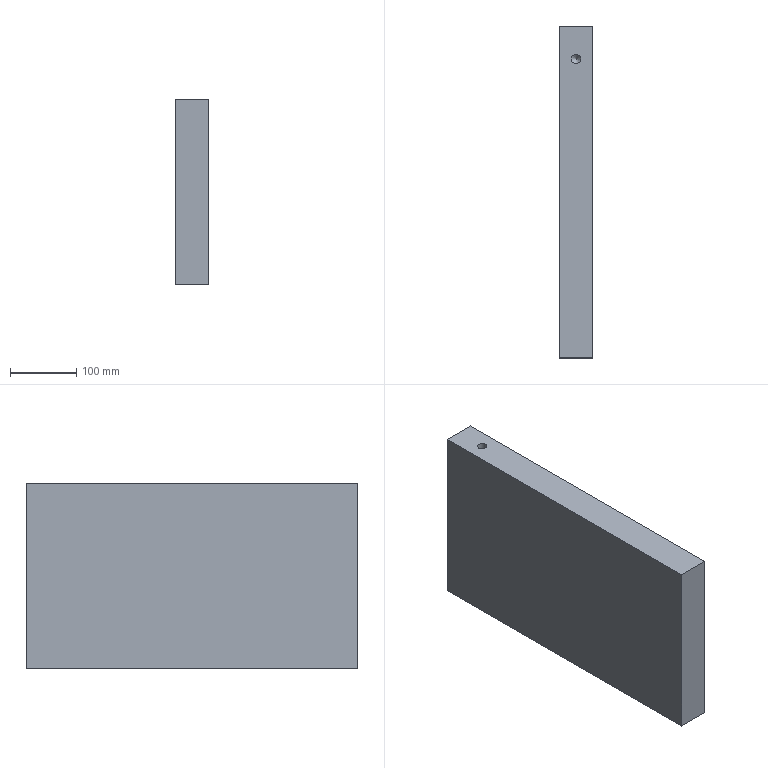Part | NX | features 29 2 | 1 solid | 12 faces | box 50 x 502.5 x 280.5 mm | volume 7029153 mm3 | plane 6 | cylinder 3 | cone 3 | commonest cylinder face diameters 14.1 x3
STEP:
#1=CARTESIAN_POINT('',(3262.05,622.5,-493.5));
#2=VERTEX_POINT('',#1);
#3=CARTESIAN_POINT('',(3255.,622.5,-493.5));
#4=DIRECTION('',(0.,0.,1.));
#5=DIRECTION('',(1.,0.,0.));
#6=AXIS2_PLACEMENT_3D('',#3,#4,#5);
#7=CIRCLE('',#6,7.05);
#8=EDGE_CURVE('',#2,#2,#7,.T.);
#9=ORIENTED_EDGE('',*,*,#8,.T.);
#10=EDGE_LOOP('',(#9));
#11=FACE_BOUND('',#10,.T.);
#12=CARTESIAN_POINT('',(3230.,170.,-493.5));
#13=VERTEX_POINT('',#12);
#14=CARTESIAN_POINT('',(3280.,170.,-493.5));
#15=VERTEX_POINT('',#14);
#16=CARTESIAN_POINT('',(1945.,170.,-493.5));
#17=DIRECTION('',(1.,0.,0.));
#18=VECTOR('',#17,1000.);
#19=LINE('',#16,#18);
#20=EDGE_CURVE('',#13,#15,#19,.T.);
#21=ORIENTED_EDGE('',*,*,#20,.F.);
#22=CARTESIAN_POINT('',(3230.,672.5,-493.5));
#23=VERTEX_POINT('',#22);
#24=CARTESIAN_POINT('',(3230.,193.,-493.5));
#25=DIRECTION('',(0.,-1.,0.));
#26=VECTOR('',#25,1000.);
#27=LINE('',#24,#26);
#28=EDGE_CURVE('',#23,#13,#27,.T.);
#29=ORIENTED_EDGE('',*,*,#28,.F.);
#30=CARTESIAN_POINT('',(3280.,672.5,-493.5));
#31=VERTEX_POINT('',#30);
#32=CARTESIAN_POINT('',(1117.5,672.5,-493.5));
#33=DIRECTION('',(1.,0.,0.));
#34=VECTOR('',#33,1000.);
#35=LINE('',#32,#34);
#36=EDGE_CURVE('',#23,#31,#35,.T.);
#37=ORIENTED_EDGE('',*,*,#36,.T.);
#38=CARTESIAN_POINT('',(3280.,193.,-493.5));
#39=DIRECTION('',(0.,1.,0.));
#40=VECTOR('',#39,1000.);
#41=LINE('',#38,#40);
#42=EDGE_CURVE('',#15,#31,#41,.T.);
#43=ORIENTED_EDGE('',*,*,#42,.F.);
#44=EDGE_LOOP('',(#21,#29,#37,#43));
#45=FACE_BOUND('',#44,.T.);
#46=CARTESIAN_POINT('',(3262.05,242.5,-493.5));
#47=VERTEX_POINT('',#46);
#48=CARTESIAN_POINT('',(3255.,242.5,-493.5));
#49=DIRECTION('',(0.,0.,1.));
#50=DIRECTION('',(1.,0.,0.));
#51=AXIS2_PLACEMENT_3D('',#48,#49,#50);
#52=CIRCLE('',#51,7.05);
#53=EDGE_CURVE('',#47,#47,#52,.T.);
#54=ORIENTED_EDGE('',*,*,#53,.T.);
#55=EDGE_LOOP('',(#54));
#56=FACE_BOUND('',#55,.T.);
#57=CARTESIAN_POINT('',(1945.,0.,-493.5));
#58=DIRECTION('',(0.,0.,-1.));
#59=DIRECTION('',(1.,0.,0.));
#60=AXIS2_PLACEMENT_3D('',#57,#58,#59);
#61=PLANE('',#60);
#62=ADVANCED_FACE('',(#11,#45,#56),#61,.T.);
#63=CARTESIAN_POINT('',(3230.,170.,-213.));
#64=VERTEX_POINT('',#63);
#65=CARTESIAN_POINT('',(3280.,170.,-213.));
#66=VERTEX_POINT('',#65);
#67=CARTESIAN_POINT('',(1945.,170.,-213.));
#68=DIRECTION('',(1.,0.,0.));
#69=VECTOR('',#68,1000.);
#70=LINE('',#67,#69);
#71=EDGE_CURVE('',#64,#66,#70,.T.);
#72=ORIENTED_EDGE('',*,*,#71,.T.);
#73=CARTESIAN_POINT('',(3280.,672.5,-213.));
#74=VERTEX_POINT('',#73);
#75=CARTESIAN_POINT('',(3280.,193.,-213.));
#76=DIRECTION('',(0.,-1.,0.));
#77=VECTOR('',#76,1000.);
#78=LINE('',#75,#77);
#79=EDGE_CURVE('',#74,#66,#78,.T.);
#80=ORIENTED_EDGE('',*,*,#79,.F.);
#81=CARTESIAN_POINT('',(3230.,672.5,-213.));
#82=VERTEX_POINT('',#81);
#83=CARTESIAN_POINT('',(1117.5,672.5,-213.));
#84=DIRECTION('',(-1.,0.,0.));
#85=VECTOR('',#84,1000.);
#86=LINE('',#83,#85);
#87=EDGE_CURVE('',#74,#82,#86,.T.);
#88=ORIENTED_EDGE('',*,*,#87,.T.);
#89=CARTESIAN_POINT('',(3230.,193.,-213.));
#90=DIRECTION('',(0.,1.,0.));
#91=VECTOR('',#90,1000.);
#92=LINE('',#89,#91);
#93=EDGE_CURVE('',#64,#82,#92,.T.);
#94=ORIENTED_EDGE('',*,*,#93,.F.);
#95=EDGE_LOOP('',(#72,#80,#88,#94));
#96=FACE_BOUND('',#95,.T.);
#97=CARTESIAN_POINT('',(3262.05,622.5,-213.));
#98=VERTEX_POINT('',#97);
#99=CARTESIAN_POINT('',(3255.,622.5,-213.));
#100=DIRECTION('',(0.,0.,-1.));
#101=DIRECTION('',(1.,0.,0.));
#102=AXIS2_PLACEMENT_3D('',#99,#100,#101);
#103=CIRCLE('',#102,7.05);
#104=EDGE_CURVE('',#98,#98,#103,.T.);
#105=ORIENTED_EDGE('',*,*,#104,.T.);
#106=EDGE_LOOP('',(#105));
#107=FACE_BOUND('',#106,.T.);
#108=CARTESIAN_POINT('',(1945.,0.,-213.));
#109=DIRECTION('',(0.,0.,1.));
#110=DIRECTION('',(-1.,0.,0.));
#111=AXIS2_PLACEMENT_3D('',#108,#109,#110);
#112=PLANE('',#111);
#113=ADVANCED_FACE('',(#96,#107),#112,.T.);
#114=CARTESIAN_POINT('',(3230.,170.,-205.5));
#115=DIRECTION('',(0.,0.,-1.));
#116=VECTOR('',#115,1000.);
#117=LINE('',#114,#116);
#118=EDGE_CURVE('',#64,#13,#117,.T.);
#119=ORIENTED_EDGE('',*,*,#118,.F.);
#120=ORIENTED_EDGE('',*,*,#93,.T.);
#121=CARTESIAN_POINT('',(3230.,672.5,-205.5));
#122=DIRECTION('',(0.,0.,1.));
#123=VECTOR('',#122,1000.);
#124=LINE('',#121,#123);
#125=EDGE_CURVE('',#23,#82,#124,.T.);
#126=ORIENTED_EDGE('',*,*,#125,.F.);
#127=ORIENTED_EDGE('',*,*,#28,.T.);
#128=EDGE_LOOP('',(#119,#120,#126,#127));
#129=FACE_BOUND('',#128,.T.);
#130=CARTESIAN_POINT('',(3230.,193.,-205.5));
#131=DIRECTION('',(-1.,0.,0.));
#132=DIRECTION('',(0.,0.,1.));
#133=AXIS2_PLACEMENT_3D('',#130,#131,#132);
#134=PLANE('',#133);
#135=ADVANCED_FACE('',(#129),#134,.T.);
#136=ORIENTED_EDGE('',*,*,#36,.F.);
#137=ORIENTED_EDGE('',*,*,#125,.T.);
#138=ORIENTED_EDGE('',*,*,#87,.F.);
#139=CARTESIAN_POINT('',(3280.,672.5,-205.5));
#140=DIRECTION('',(0.,0.,1.));
#141=VECTOR('',#140,1000.);
#142=LINE('',#139,#141);
#143=EDGE_CURVE('',#31,#74,#142,.T.);
#144=ORIENTED_EDGE('',*,*,#143,.F.);
#145=EDGE_LOOP('',(#136,#137,#138,#144));
#146=FACE_BOUND('',#145,.T.);
#147=CARTESIAN_POINT('',(1117.5,672.5,91.));
#148=DIRECTION('',(0.,-1.,0.));
#149=DIRECTION('',(-1.,0.,0.));
#150=AXIS2_PLACEMENT_3D('',#147,#148,#149);
#151=PLANE('',#150);
#152=ADVANCED_FACE('',(#146),#151,.F.);
#153=CARTESIAN_POINT('',(3280.,170.,-205.5));
#154=DIRECTION('',(0.,0.,-1.));
#155=VECTOR('',#154,1000.);
#156=LINE('',#153,#155);
#157=EDGE_CURVE('',#66,#15,#156,.T.);
#158=ORIENTED_EDGE('',*,*,#157,.T.);
#159=ORIENTED_EDGE('',*,*,#42,.T.);
#160=ORIENTED_EDGE('',*,*,#143,.T.);
#161=ORIENTED_EDGE('',*,*,#79,.T.);
#162=EDGE_LOOP('',(#158,#159,#160,#161));
#163=FACE_BOUND('',#162,.T.);
#164=CARTESIAN_POINT('',(3280.,193.,-205.5));
#165=DIRECTION('',(1.,0.,0.));
#166=DIRECTION('',(0.,0.,-1.));
#167=AXIS2_PLACEMENT_3D('',#164,#165,#166);
#168=PLANE('',#167);
#169=ADVANCED_FACE('',(#163),#168,.T.);
#170=ORIENTED_EDGE('',*,*,#71,.F.);
#171=ORIENTED_EDGE('',*,*,#118,.T.);
#172=ORIENTED_EDGE('',*,*,#20,.T.);
#173=ORIENTED_EDGE('',*,*,#157,.F.);
#174=EDGE_LOOP('',(#170,#171,#172,#173));
#175=FACE_BOUND('',#174,.T.);
#176=CARTESIAN_POINT('',(2874.,170.,0.));
#177=DIRECTION('',(0.,1.,0.));
#178=DIRECTION('',(0.,0.,-1.));
#179=AXIS2_PLACEMENT_3D('',#176,#177,#178);
#180=PLANE('',#179);
#181=ADVANCED_FACE('',(#175),#180,.F.);
#182=CARTESIAN_POINT('',(3247.95,622.5,-249.95));
#183=VERTEX_POINT('',#182);
#184=CARTESIAN_POINT('',(3255.,622.5,-249.95));
#185=DIRECTION('',(0.,0.,-1.));
#186=DIRECTION('',(-1.,0.,0.));
#187=AXIS2_PLACEMENT_3D('',#184,#185,#186);
#188=CIRCLE('',#187,7.05);
#189=EDGE_CURVE('',#183,#183,#188,.T.);
#190=ORIENTED_EDGE('',*,*,#189,.T.);
#191=EDGE_LOOP('',(#190));
#192=FACE_BOUND('',#191,.T.);
#193=ORIENTED_EDGE('',*,*,#104,.F.);
#194=EDGE_LOOP('',(#193));
#195=FACE_BOUND('',#194,.T.);
#196=CARTESIAN_POINT('',(3255.,622.5,-213.));
#197=DIRECTION('',(0.,0.,-1.));
#198=DIRECTION('',(-1.,0.,0.));
#199=AXIS2_PLACEMENT_3D('',#196,#197,#198);
#200=CYLINDRICAL_SURFACE('',#199,7.05);
#201=ADVANCED_FACE('',(#192,#195),#200,.F.);
#202=CARTESIAN_POINT('',(3255.,622.5,-257.));
#203=VERTEX_POINT('',#202);
#204=VERTEX_LOOP('',#203);
#205=FACE_BOUND('',#204,.T.);
#206=ORIENTED_EDGE('',*,*,#189,.F.);
#207=EDGE_LOOP('',(#206));
#208=FACE_BOUND('',#207,.T.);
#209=CARTESIAN_POINT('',(3255.,622.5,-249.95));
#210=DIRECTION('',(0.,0.,1.));
#211=DIRECTION('',(-1.,0.,0.));
#212=AXIS2_PLACEMENT_3D('',#209,#210,#211);
#213=CONICAL_SURFACE('',#212,7.05,0.7854);
#214=ADVANCED_FACE('',(#205,#208),#213,.F.);
#215=CARTESIAN_POINT('',(3262.05,622.5,-456.55));
#216=VERTEX_POINT('',#215);
#217=CARTESIAN_POINT('',(3255.,622.5,-456.55));
#218=DIRECTION('',(0.,0.,1.));
#219=DIRECTION('',(1.,0.,0.));
#220=AXIS2_PLACEMENT_3D('',#217,#218,#219);
#221=CIRCLE('',#220,7.05);
#222=EDGE_CURVE('',#216,#216,#221,.T.);
#223=ORIENTED_EDGE('',*,*,#222,.T.);
#224=EDGE_LOOP('',(#223));
#225=FACE_BOUND('',#224,.T.);
#226=ORIENTED_EDGE('',*,*,#8,.F.);
#227=EDGE_LOOP('',(#226));
#228=FACE_BOUND('',#227,.T.);
#229=CARTESIAN_POINT('',(3255.,622.5,-493.5));
#230=DIRECTION('',(0.,0.,1.));
#231=DIRECTION('',(-1.,0.,0.));
#232=AXIS2_PLACEMENT_3D('',#229,#230,#231);
#233=CYLINDRICAL_SURFACE('',#232,7.05);
#234=ADVANCED_FACE('',(#225,#228),#233,.F.);
#235=CARTESIAN_POINT('',(3255.,622.5,-449.5));
#236=VERTEX_POINT('',#235);
#237=VERTEX_LOOP('',#236);
#238=FACE_BOUND('',#237,.T.);
#239=ORIENTED_EDGE('',*,*,#222,.F.);
#240=EDGE_LOOP('',(#239));
#241=FACE_BOUND('',#240,.T.);
#242=CARTESIAN_POINT('',(3255.,622.5,-456.55));
#243=DIRECTION('',(0.,0.,-1.));
#244=DIRECTION('',(1.,0.,0.));
#245=AXIS2_PLACEMENT_3D('',#242,#243,#244);
#246=CONICAL_SURFACE('',#245,7.05,0.7854);
#247=ADVANCED_FACE('',(#238,#241),#246,.F.);
#248=CARTESIAN_POINT('',(3262.05,242.5,-456.55));
#249=VERTEX_POINT('',#248);
#250=CARTESIAN_POINT('',(3255.,242.5,-456.55));
#251=DIRECTION('',(0.,0.,1.));
#252=DIRECTION('',(1.,0.,0.));
#253=AXIS2_PLACEMENT_3D('',#250,#251,#252);
#254=CIRCLE('',#253,7.05);
#255=EDGE_CURVE('',#249,#249,#254,.T.);
#256=ORIENTED_EDGE('',*,*,#255,.T.);
#257=EDGE_LOOP('',(#256));
#258=FACE_BOUND('',#257,.T.);
#259=ORIENTED_EDGE('',*,*,#53,.F.);
#260=EDGE_LOOP('',(#259));
#261=FACE_BOUND('',#260,.T.);
#262=CARTESIAN_POINT('',(3255.,242.5,-493.5));
#263=DIRECTION('',(0.,0.,1.));
#264=DIRECTION('',(-1.,0.,0.));
#265=AXIS2_PLACEMENT_3D('',#262,#263,#264);
#266=CYLINDRICAL_SURFACE('',#265,7.05);
#267=ADVANCED_FACE('',(#258,#261),#266,.F.);
#268=CARTESIAN_POINT('',(3255.,242.5,-449.5));
#269=VERTEX_POINT('',#268);
#270=VERTEX_LOOP('',#269);
#271=FACE_BOUND('',#270,.T.);
#272=ORIENTED_EDGE('',*,*,#255,.F.);
#273=EDGE_LOOP('',(#272));
#274=FACE_BOUND('',#273,.T.);
#275=CARTESIAN_POINT('',(3255.,242.5,-456.55));
#276=DIRECTION('',(0.,0.,-1.));
#277=DIRECTION('',(1.,0.,0.));
#278=AXIS2_PLACEMENT_3D('',#275,#276,#277);
#279=CONICAL_SURFACE('',#278,7.05,0.7854);
#280=ADVANCED_FACE('',(#271,#274),#279,.F.);
#281=CLOSED_SHELL('',(#62,#113,#135,#152,#169,#181,#201,#214,#234,#247,#267,#280));
#282=MANIFOLD_SOLID_BREP('',#281);
#283=(LENGTH_UNIT()NAMED_UNIT(*)SI_UNIT(.MILLI.,.METRE.));
#284=UNCERTAINTY_MEASURE_WITH_UNIT(LENGTH_MEASURE(0.00001),#283,'','');
#285=(NAMED_UNIT(*)PLANE_ANGLE_UNIT()SI_UNIT($,.RADIAN.));
#286=(NAMED_UNIT(*)SI_UNIT($,.STERADIAN.)SOLID_ANGLE_UNIT());
#287=(GEOMETRIC_REPRESENTATION_CONTEXT(3)GLOBAL_UNCERTAINTY_ASSIGNED_CONTEXT((#284))GLOBAL_UNIT_ASSIGNED_CONTEXT((#283,#285,#286))REPRESENTATION_CONTEXT('',''));
#288=ADVANCED_BREP_SHAPE_REPRESENTATION('',(#282),#287);